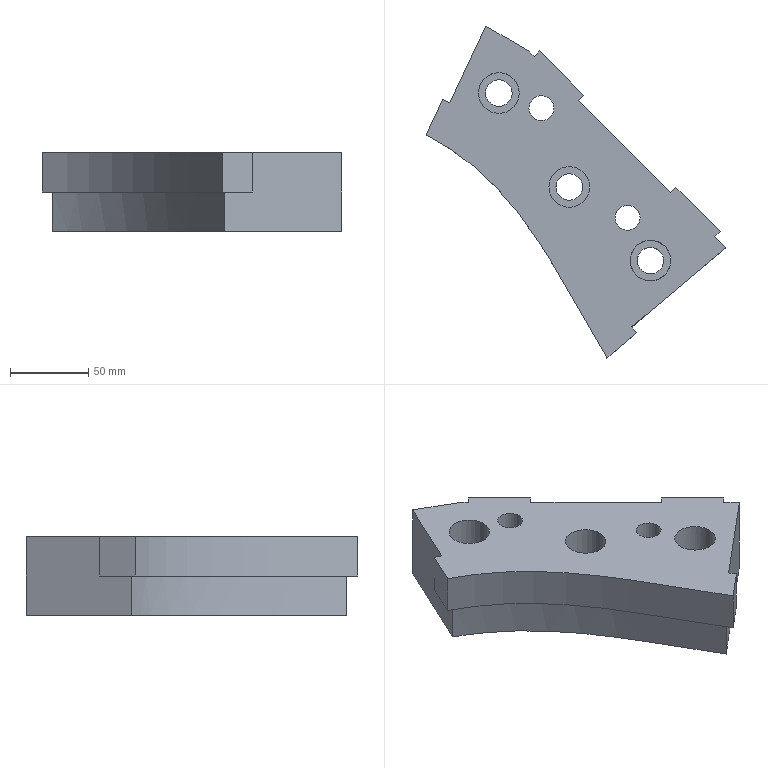Part | NX | features solid 2 | 1 solid | 32 faces | box 191.378 x 212.047 x 50 mm | volume 733271 mm3 | plane 22 | cylinder 8 | spline 2 | commonest cylinder face diameters 17 x3 26 x3 16 x2
STEP:
#1=CARTESIAN_POINT('',(8.245,-336.739,0.));
#2=VERTEX_POINT('',#1);
#3=CARTESIAN_POINT('',(1.173,-329.668,0.));
#4=VERTEX_POINT('',#3);
#5=CARTESIAN_POINT('',(11.794,-340.288,0.));
#6=DIRECTION('',(-0.7071,0.7071,0.));
#7=VECTOR('',#6,1000.);
#8=LINE('',#5,#7);
#9=EDGE_CURVE('',#2,#4,#8,.T.);
#10=ORIENTED_EDGE('',*,*,#9,.F.);
#11=CARTESIAN_POINT('',(8.245,-336.739,-50.));
#12=VERTEX_POINT('',#11);
#13=CARTESIAN_POINT('',(8.245,-336.739,-50.));
#14=DIRECTION('',(0.,0.,1.));
#15=VECTOR('',#14,1000.);
#16=LINE('',#13,#15);
#17=EDGE_CURVE('',#12,#2,#16,.T.);
#18=ORIENTED_EDGE('',*,*,#17,.F.);
#19=CARTESIAN_POINT('',(1.173,-329.668,-50.));
#20=VERTEX_POINT('',#19);
#21=CARTESIAN_POINT('',(11.794,-340.288,-50.));
#22=DIRECTION('',(-0.7071,0.7071,0.));
#23=VECTOR('',#22,1000.);
#24=LINE('',#21,#23);
#25=EDGE_CURVE('',#12,#20,#24,.T.);
#26=ORIENTED_EDGE('',*,*,#25,.T.);
#27=CARTESIAN_POINT('',(1.173,-329.668,-50.));
#28=DIRECTION('',(0.,0.,1.));
#29=VECTOR('',#28,1000.);
#30=LINE('',#27,#29);
#31=EDGE_CURVE('',#20,#4,#30,.T.);
#32=ORIENTED_EDGE('',*,*,#31,.T.);
#33=EDGE_LOOP('',(#10,#18,#26,#32));
#34=FACE_BOUND('',#33,.T.);
#35=CARTESIAN_POINT('',(11.794,-340.288,-50.));
#36=DIRECTION('',(0.7071,0.7071,0.));
#37=DIRECTION('',(-0.7071,0.7071,0.));
#38=AXIS2_PLACEMENT_3D('',#35,#36,#37);
#39=PLANE('',#38);
#40=ADVANCED_FACE('',(#34),#39,.T.);
#41=CARTESIAN_POINT('',(-48.541,-390.915,-25.));
#42=VERTEX_POINT('',#41);
#43=CARTESIAN_POINT('',(-51.755,-387.085,-25.));
#44=VERTEX_POINT('',#43);
#45=CARTESIAN_POINT('',(-45.327,-394.745,-25.));
#46=DIRECTION('',(-0.6428,0.766,0.));
#47=VECTOR('',#46,1000.);
#48=LINE('',#45,#47);
#49=EDGE_CURVE('',#42,#44,#48,.T.);
#50=ORIENTED_EDGE('',*,*,#49,.F.);
#51=CARTESIAN_POINT('',(-67.692,-406.985,-25.));
#52=VERTEX_POINT('',#51);
#53=CARTESIAN_POINT('',(-67.692,-406.985,-25.));
#54=DIRECTION('',(-0.766,-0.6428,0.));
#55=VECTOR('',#54,1000.);
#56=LINE('',#53,#55);
#57=EDGE_CURVE('',#42,#52,#56,.T.);
#58=ORIENTED_EDGE('',*,*,#57,.T.);
#59=CARTESIAN_POINT('',(-183.133,-264.552,-25.));
#60=VERTEX_POINT('',#59);
#61=CARTESIAN_POINT('',(-183.133,-264.552,-25.));
#62=CARTESIAN_POINT('',(-182.734,-264.756,-25.));
#63=CARTESIAN_POINT('',(-176.179,-268.157,-25.));
#64=CARTESIAN_POINT('',(-163.887,-275.581,-25.));
#65=CARTESIAN_POINT('',(-147.555,-288.567,-25.));
#66=CARTESIAN_POINT('',(-132.971,-303.448,-25.));
#67=CARTESIAN_POINT('',(-115.628,-325.186,-25.));
#68=CARTESIAN_POINT('',(-97.34,-354.727,-25.));
#69=CARTESIAN_POINT('',(-80.928,-384.396,-25.));
#70=CARTESIAN_POINT('',(-70.839,-401.701,-25.));
#71=CARTESIAN_POINT('',(-67.692,-406.985,-25.));
#72=B_SPLINE_CURVE_WITH_KNOTS('',3,(#61,#62,#63,#64,#65,#66,#67,#68,#69,#70,#71),.UNSPECIFIED.,.F.,.F.,(4,1,1,1,1,1,1,1,4),(0.,0.007224,0.1189,0.2307,0.3424,0.4541,0.6776,0.901,1.),.UNSPECIFIED.);
#73=EDGE_CURVE('',#52,#60,#72,.F.);
#74=ORIENTED_EDGE('',*,*,#73,.T.);
#75=CARTESIAN_POINT('',(-172.568,-241.894,-25.));
#76=VERTEX_POINT('',#75);
#77=CARTESIAN_POINT('',(-183.133,-264.552,-25.));
#78=DIRECTION('',(-0.4226,-0.9063,0.));
#79=VECTOR('',#78,1000.);
#80=LINE('',#77,#79);
#81=EDGE_CURVE('',#76,#60,#80,.T.);
#82=ORIENTED_EDGE('',*,*,#81,.F.);
#83=CARTESIAN_POINT('',(-168.036,-244.007,-25.));
#84=VERTEX_POINT('',#83);
#85=CARTESIAN_POINT('',(-177.099,-239.781,-25.));
#86=DIRECTION('',(0.9063,-0.4226,0.));
#87=VECTOR('',#86,1000.);
#88=LINE('',#85,#87);
#89=EDGE_CURVE('',#76,#84,#88,.T.);
#90=ORIENTED_EDGE('',*,*,#89,.T.);
#91=CARTESIAN_POINT('',(-176.596,-262.363,-25.));
#92=VERTEX_POINT('',#91);
#93=CARTESIAN_POINT('',(-178.602,-266.665,-25.));
#94=DIRECTION('',(-0.4226,-0.9063,0.));
#95=VECTOR('',#94,1000.);
#96=LINE('',#93,#95);
#97=EDGE_CURVE('',#92,#84,#96,.F.);
#98=ORIENTED_EDGE('',*,*,#97,.F.);
#99=CARTESIAN_POINT('',(-66.391,-399.365,-25.));
#100=VERTEX_POINT('',#99);
#101=CARTESIAN_POINT('',(-176.596,-262.363,-25.));
#102=CARTESIAN_POINT('',(-169.988,-265.991,-25.));
#103=CARTESIAN_POINT('',(-157.223,-274.12,-25.));
#104=CARTESIAN_POINT('',(-134.139,-293.687,-25.));
#105=CARTESIAN_POINT('',(-110.503,-323.019,-25.));
#106=CARTESIAN_POINT('',(-87.959,-361.257,-25.));
#107=CARTESIAN_POINT('',(-73.779,-386.798,-25.));
#108=CARTESIAN_POINT('',(-66.391,-399.365,-25.));
#109=B_SPLINE_CURVE_WITH_KNOTS('',3,(#101,#102,#103,#104,#105,#106,#107,#108),.UNSPECIFIED.,.F.,.F.,(4,1,1,1,1,4),(0.02511,0.143,0.2609,0.4967,0.7325,0.9683),.UNSPECIFIED.);
#110=EDGE_CURVE('',#92,#100,#109,.T.);
#111=ORIENTED_EDGE('',*,*,#110,.T.);
#112=CARTESIAN_POINT('',(-70.906,-403.154,-25.));
#113=DIRECTION('',(-0.766,-0.6428,0.));
#114=VECTOR('',#113,1000.);
#115=LINE('',#112,#114);
#116=EDGE_CURVE('',#100,#44,#115,.F.);
#117=ORIENTED_EDGE('',*,*,#116,.T.);
#118=EDGE_LOOP('',(#50,#58,#74,#82,#90,#98,#111,#117));
#119=FACE_BOUND('',#118,.T.);
#120=CARTESIAN_POINT('',(-56.169,-397.653,-25.));
#121=DIRECTION('',(0.,0.,-1.));
#122=DIRECTION('',(-1.,0.,0.));
#123=AXIS2_PLACEMENT_3D('',#120,#121,#122);
#124=PLANE('',#123);
#125=ADVANCED_FACE('',(#119),#124,.T.);
#126=CARTESIAN_POINT('',(-101.523,-247.421,0.));
#127=VERTEX_POINT('',#126);
#128=CARTESIAN_POINT('',(-109.523,-247.421,0.));
#129=DIRECTION('',(0.,0.,1.));
#130=DIRECTION('',(1.,0.,0.));
#131=AXIS2_PLACEMENT_3D('',#128,#129,#130);
#132=CIRCLE('',#131,8.);
#133=EDGE_CURVE('',#127,#127,#132,.T.);
#134=ORIENTED_EDGE('',*,*,#133,.F.);
#135=EDGE_LOOP('',(#134));
#136=FACE_BOUND('',#135,.T.);
#137=CARTESIAN_POINT('',(-46.523,-317.421,0.));
#138=VERTEX_POINT('',#137);
#139=CARTESIAN_POINT('',(-54.523,-317.421,0.));
#140=DIRECTION('',(0.,0.,1.));
#141=DIRECTION('',(1.,0.,0.));
#142=AXIS2_PLACEMENT_3D('',#139,#140,#141);
#143=CIRCLE('',#142,8.);
#144=EDGE_CURVE('',#138,#138,#143,.T.);
#145=ORIENTED_EDGE('',*,*,#144,.F.);
#146=EDGE_LOOP('',(#145));
#147=FACE_BOUND('',#146,.T.);
#148=CARTESIAN_POINT('',(-48.541,-390.915,0.));
#149=VERTEX_POINT('',#148);
#150=CARTESIAN_POINT('',(-51.755,-387.085,0.));
#151=VERTEX_POINT('',#150);
#152=CARTESIAN_POINT('',(-45.327,-394.745,0.));
#153=DIRECTION('',(-0.6428,0.766,0.));
#154=VECTOR('',#153,1000.);
#155=LINE('',#152,#154);
#156=EDGE_CURVE('',#149,#151,#155,.T.);
#157=ORIENTED_EDGE('',*,*,#156,.T.);
#158=CARTESIAN_POINT('',(-70.906,-403.154,0.));
#159=DIRECTION('',(0.766,0.6428,0.));
#160=VECTOR('',#159,1000.);
#161=LINE('',#158,#160);
#162=EDGE_CURVE('',#151,#2,#161,.T.);
#163=ORIENTED_EDGE('',*,*,#162,.T.);
#164=ORIENTED_EDGE('',*,*,#9,.T.);
#165=CARTESIAN_POINT('',(4.709,-326.132,0.));
#166=VERTEX_POINT('',#165);
#167=CARTESIAN_POINT('',(1.173,-329.668,0.));
#168=DIRECTION('',(0.7071,0.7071,0.));
#169=VECTOR('',#168,1000.);
#170=LINE('',#167,#169);
#171=EDGE_CURVE('',#4,#166,#170,.T.);
#172=ORIENTED_EDGE('',*,*,#171,.T.);
#173=CARTESIAN_POINT('',(-23.575,-297.848,0.));
#174=VERTEX_POINT('',#173);
#175=CARTESIAN_POINT('',(109.467,-430.891,0.));
#176=DIRECTION('',(-0.7071,0.7071,0.));
#177=VECTOR('',#176,1000.);
#178=LINE('',#175,#177);
#179=EDGE_CURVE('',#166,#174,#178,.T.);
#180=ORIENTED_EDGE('',*,*,#179,.T.);
#181=CARTESIAN_POINT('',(-27.111,-301.384,0.));
#182=VERTEX_POINT('',#181);
#183=CARTESIAN_POINT('',(-27.111,-301.384,0.));
#184=DIRECTION('',(0.7071,0.7071,0.));
#185=VECTOR('',#184,1000.);
#186=LINE('',#183,#185);
#187=EDGE_CURVE('',#182,#174,#186,.T.);
#188=ORIENTED_EDGE('',*,*,#187,.F.);
#189=CARTESIAN_POINT('',(-85.894,-242.601,0.));
#190=VERTEX_POINT('',#189);
#191=CARTESIAN_POINT('',(11.794,-340.288,0.));
#192=DIRECTION('',(-0.7071,0.7071,0.));
#193=VECTOR('',#192,1000.);
#194=LINE('',#191,#193);
#195=EDGE_CURVE('',#182,#190,#194,.T.);
#196=ORIENTED_EDGE('',*,*,#195,.T.);
#197=CARTESIAN_POINT('',(-82.358,-239.065,0.));
#198=VERTEX_POINT('',#197);
#199=CARTESIAN_POINT('',(-85.894,-242.601,0.));
#200=DIRECTION('',(0.7071,0.7071,0.));
#201=VECTOR('',#200,1000.);
#202=LINE('',#199,#201);
#203=EDGE_CURVE('',#190,#198,#202,.T.);
#204=ORIENTED_EDGE('',*,*,#203,.T.);
#205=CARTESIAN_POINT('',(-110.642,-210.781,0.));
#206=VERTEX_POINT('',#205);
#207=CARTESIAN_POINT('',(15.329,-336.753,0.));
#208=DIRECTION('',(-0.7071,0.7071,0.));
#209=VECTOR('',#208,1000.);
#210=LINE('',#207,#209);
#211=EDGE_CURVE('',#198,#206,#210,.T.);
#212=ORIENTED_EDGE('',*,*,#211,.T.);
#213=CARTESIAN_POINT('',(-114.178,-214.317,0.));
#214=VERTEX_POINT('',#213);
#215=CARTESIAN_POINT('',(-114.178,-214.317,0.));
#216=DIRECTION('',(0.7071,0.7071,0.));
#217=VECTOR('',#216,1000.);
#218=LINE('',#215,#217);
#219=EDGE_CURVE('',#214,#206,#218,.T.);
#220=ORIENTED_EDGE('',*,*,#219,.F.);
#221=CARTESIAN_POINT('',(-117.713,-210.781,0.));
#222=VERTEX_POINT('',#221);
#223=CARTESIAN_POINT('',(11.794,-340.288,0.));
#224=DIRECTION('',(-0.7071,0.7071,0.));
#225=VECTOR('',#224,1000.);
#226=LINE('',#223,#225);
#227=EDGE_CURVE('',#214,#222,#226,.T.);
#228=ORIENTED_EDGE('',*,*,#227,.T.);
#229=CARTESIAN_POINT('',(-145.155,-194.938,0.));
#230=VERTEX_POINT('',#229);
#231=CARTESIAN_POINT('',(-65.584,-240.878,0.));
#232=DIRECTION('',(-0.866,0.5,0.));
#233=VECTOR('',#232,1000.);
#234=LINE('',#231,#233);
#235=EDGE_CURVE('',#222,#230,#234,.T.);
#236=ORIENTED_EDGE('',*,*,#235,.T.);
#237=CARTESIAN_POINT('',(-168.036,-244.007,0.));
#238=VERTEX_POINT('',#237);
#239=CARTESIAN_POINT('',(-178.602,-266.665,0.));
#240=DIRECTION('',(0.4226,0.9063,0.));
#241=VECTOR('',#240,1000.);
#242=LINE('',#239,#241);
#243=EDGE_CURVE('',#238,#230,#242,.T.);
#244=ORIENTED_EDGE('',*,*,#243,.F.);
#245=CARTESIAN_POINT('',(-172.568,-241.894,0.));
#246=VERTEX_POINT('',#245);
#247=CARTESIAN_POINT('',(-177.099,-239.781,0.));
#248=DIRECTION('',(0.9063,-0.4226,0.));
#249=VECTOR('',#248,1000.);
#250=LINE('',#247,#249);
#251=EDGE_CURVE('',#246,#238,#250,.T.);
#252=ORIENTED_EDGE('',*,*,#251,.F.);
#253=CARTESIAN_POINT('',(-183.133,-264.552,0.));
#254=VERTEX_POINT('',#253);
#255=CARTESIAN_POINT('',(-183.133,-264.552,0.));
#256=DIRECTION('',(0.4226,0.9063,0.));
#257=VECTOR('',#256,1000.);
#258=LINE('',#255,#257);
#259=EDGE_CURVE('',#254,#246,#258,.T.);
#260=ORIENTED_EDGE('',*,*,#259,.F.);
#261=CARTESIAN_POINT('',(-67.692,-406.985,0.));
#262=VERTEX_POINT('',#261);
#263=CARTESIAN_POINT('',(-183.133,-264.552,0.));
#264=CARTESIAN_POINT('',(-182.734,-264.756,0.));
#265=CARTESIAN_POINT('',(-176.179,-268.157,0.));
#266=CARTESIAN_POINT('',(-163.887,-275.581,0.));
#267=CARTESIAN_POINT('',(-147.555,-288.567,0.));
#268=CARTESIAN_POINT('',(-132.971,-303.448,0.));
#269=CARTESIAN_POINT('',(-115.628,-325.186,0.));
#270=CARTESIAN_POINT('',(-97.34,-354.727,0.));
#271=CARTESIAN_POINT('',(-80.928,-384.396,0.));
#272=CARTESIAN_POINT('',(-70.839,-401.701,0.));
#273=CARTESIAN_POINT('',(-67.692,-406.985,0.));
#274=B_SPLINE_CURVE_WITH_KNOTS('',3,(#263,#264,#265,#266,#267,#268,#269,#270,#271,#272,#273),.UNSPECIFIED.,.F.,.F.,(4,1,1,1,1,1,1,1,4),(0.,0.007224,0.1189,0.2307,0.3424,0.4541,0.6776,0.901,1.),.UNSPECIFIED.);
#275=EDGE_CURVE('',#254,#262,#274,.T.);
#276=ORIENTED_EDGE('',*,*,#275,.T.);
#277=CARTESIAN_POINT('',(-67.692,-406.985,0.));
#278=DIRECTION('',(0.766,0.6428,0.));
#279=VECTOR('',#278,1000.);
#280=LINE('',#277,#279);
#281=EDGE_CURVE('',#262,#149,#280,.T.);
#282=ORIENTED_EDGE('',*,*,#281,.T.);
#283=EDGE_LOOP('',(#157,#163,#164,#172,#180,#188,#196,#204,#212,#220,#228,#236,#244,#252,#260,#276,#282));
#284=FACE_BOUND('',#283,.T.);
#285=CARTESIAN_POINT('',(-78.729,-297.741,0.));
#286=VERTEX_POINT('',#285);
#287=CARTESIAN_POINT('',(-91.729,-297.741,0.));
#288=DIRECTION('',(0.,0.,1.));
#289=DIRECTION('',(1.,0.,0.));
#290=AXIS2_PLACEMENT_3D('',#287,#288,#289);
#291=CIRCLE('',#290,13.);
#292=EDGE_CURVE('',#286,#286,#291,.T.);
#293=ORIENTED_EDGE('',*,*,#292,.F.);
#294=EDGE_LOOP('',(#293));
#295=FACE_BOUND('',#294,.T.);
#296=CARTESIAN_POINT('',(-26.878,-344.794,0.));
#297=VERTEX_POINT('',#296);
#298=CARTESIAN_POINT('',(-39.878,-344.794,0.));
#299=DIRECTION('',(0.,0.,1.));
#300=DIRECTION('',(1.,0.,0.));
#301=AXIS2_PLACEMENT_3D('',#298,#299,#300);
#302=CIRCLE('',#301,13.);
#303=EDGE_CURVE('',#297,#297,#302,.T.);
#304=ORIENTED_EDGE('',*,*,#303,.F.);
#305=EDGE_LOOP('',(#304));
#306=FACE_BOUND('',#305,.T.);
#307=CARTESIAN_POINT('',(-123.729,-237.741,0.));
#308=VERTEX_POINT('',#307);
#309=CARTESIAN_POINT('',(-136.729,-237.741,0.));
#310=DIRECTION('',(0.,0.,1.));
#311=DIRECTION('',(1.,0.,0.));
#312=AXIS2_PLACEMENT_3D('',#309,#310,#311);
#313=CIRCLE('',#312,13.);
#314=EDGE_CURVE('',#308,#308,#313,.T.);
#315=ORIENTED_EDGE('',*,*,#314,.F.);
#316=EDGE_LOOP('',(#315));
#317=FACE_BOUND('',#316,.T.);
#318=CARTESIAN_POINT('',(-557.805,-998.377,0.));
#319=DIRECTION('',(0.,0.,1.));
#320=DIRECTION('',(1.,0.,0.));
#321=AXIS2_PLACEMENT_3D('',#318,#319,#320);
#322=PLANE('',#321);
#323=ADVANCED_FACE('',(#136,#147,#284,#295,#306,#317),#322,.T.);
#324=CARTESIAN_POINT('',(-172.568,-241.894,-50.));
#325=DIRECTION('',(0.,0.,1.));
#326=VECTOR('',#325,1000.);
#327=LINE('',#324,#326);
#328=EDGE_CURVE('',#76,#246,#327,.T.);
#329=ORIENTED_EDGE('',*,*,#328,.F.);
#330=ORIENTED_EDGE('',*,*,#81,.T.);
#331=CARTESIAN_POINT('',(-183.133,-264.552,-50.));
#332=DIRECTION('',(0.,0.,1.));
#333=VECTOR('',#332,1000.);
#334=LINE('',#331,#333);
#335=EDGE_CURVE('',#60,#254,#334,.T.);
#336=ORIENTED_EDGE('',*,*,#335,.T.);
#337=ORIENTED_EDGE('',*,*,#259,.T.);
#338=EDGE_LOOP('',(#329,#330,#336,#337));
#339=FACE_BOUND('',#338,.T.);
#340=CARTESIAN_POINT('',(-183.133,-264.552,-50.));
#341=DIRECTION('',(0.9063,-0.4226,0.));
#342=DIRECTION('',(0.4226,0.9063,0.));
#343=AXIS2_PLACEMENT_3D('',#340,#341,#342);
#344=PLANE('',#343);
#345=ADVANCED_FACE('',(#339),#344,.F.);
#346=CARTESIAN_POINT('',(-101.523,-247.421,-50.));
#347=VERTEX_POINT('',#346);
#348=CARTESIAN_POINT('',(-109.523,-247.421,-50.));
#349=DIRECTION('',(0.,0.,1.));
#350=DIRECTION('',(1.,0.,0.));
#351=AXIS2_PLACEMENT_3D('',#348,#349,#350);
#352=CIRCLE('',#351,8.);
#353=EDGE_CURVE('',#347,#347,#352,.T.);
#354=ORIENTED_EDGE('',*,*,#353,.T.);
#355=EDGE_LOOP('',(#354));
#356=FACE_BOUND('',#355,.T.);
#357=CARTESIAN_POINT('',(-46.523,-317.421,-50.));
#358=VERTEX_POINT('',#357);
#359=CARTESIAN_POINT('',(-54.523,-317.421,-50.));
#360=DIRECTION('',(0.,0.,1.));
#361=DIRECTION('',(1.,0.,0.));
#362=AXIS2_PLACEMENT_3D('',#359,#360,#361);
#363=CIRCLE('',#362,8.);
#364=EDGE_CURVE('',#358,#358,#363,.T.);
#365=ORIENTED_EDGE('',*,*,#364,.T.);
#366=EDGE_LOOP('',(#365));
#367=FACE_BOUND('',#366,.T.);
#368=CARTESIAN_POINT('',(-128.229,-237.741,-50.));
#369=VERTEX_POINT('',#368);
#370=CARTESIAN_POINT('',(-136.729,-237.741,-50.));
#371=DIRECTION('',(0.,0.,1.));
#372=DIRECTION('',(1.,0.,0.));
#373=AXIS2_PLACEMENT_3D('',#370,#371,#372);
#374=CIRCLE('',#373,8.5);
#375=EDGE_CURVE('',#369,#369,#374,.T.);
#376=ORIENTED_EDGE('',*,*,#375,.T.);
#377=EDGE_LOOP('',(#376));
#378=FACE_BOUND('',#377,.T.);
#379=ORIENTED_EDGE('',*,*,#25,.F.);
#380=CARTESIAN_POINT('',(-66.391,-399.365,-50.));
#381=VERTEX_POINT('',#380);
#382=CARTESIAN_POINT('',(-59.36,-393.466,-50.));
#383=DIRECTION('',(-0.766,-0.6428,0.));
#384=VECTOR('',#383,1000.);
#385=LINE('',#382,#384);
#386=EDGE_CURVE('',#12,#381,#385,.T.);
#387=ORIENTED_EDGE('',*,*,#386,.T.);
#388=CARTESIAN_POINT('',(-176.596,-262.363,-50.));
#389=VERTEX_POINT('',#388);
#390=CARTESIAN_POINT('',(-66.391,-399.365,-50.));
#391=CARTESIAN_POINT('',(-67.194,-397.999,-50.));
#392=CARTESIAN_POINT('',(-68.864,-395.141,-50.));
#393=CARTESIAN_POINT('',(-71.109,-391.26,-50.));
#394=CARTESIAN_POINT('',(-73.001,-387.969,-50.));
#395=CARTESIAN_POINT('',(-74.222,-385.835,-50.));
#396=CARTESIAN_POINT('',(-75.223,-384.08,-50.));
#397=CARTESIAN_POINT('',(-75.984,-382.743,-50.));
#398=CARTESIAN_POINT('',(-76.633,-381.601,-50.));
#399=CARTESIAN_POINT('',(-77.082,-380.81,-50.));
#400=CARTESIAN_POINT('',(-77.357,-380.325,-50.));
#401=CARTESIAN_POINT('',(-77.517,-380.043,-50.));
#402=CARTESIAN_POINT('',(-77.857,-379.443,-50.));
#403=CARTESIAN_POINT('',(-78.241,-378.766,-50.));
#404=CARTESIAN_POINT('',(-78.929,-377.553,-50.));
#405=CARTESIAN_POINT('',(-79.854,-375.92,-50.));
#406=CARTESIAN_POINT('',(-80.906,-374.065,-50.));
#407=CARTESIAN_POINT('',(-82.219,-371.751,-50.));
#408=CARTESIAN_POINT('',(-83.697,-369.146,-50.));
#409=CARTESIAN_POINT('',(-85.208,-366.484,-50.));
#410=CARTESIAN_POINT('',(-86.457,-364.285,-50.));
#411=CARTESIAN_POINT('',(-87.278,-362.839,-50.));
#412=CARTESIAN_POINT('',(-87.805,-361.914,-50.));
#413=CARTESIAN_POINT('',(-88.079,-361.433,-50.));
#414=CARTESIAN_POINT('',(-88.266,-361.105,-50.));
#415=CARTESIAN_POINT('',(-88.389,-360.89,-50.));
#416=CARTESIAN_POINT('',(-88.482,-360.728,-50.));
#417=CARTESIAN_POINT('',(-88.531,-360.641,-50.));
#418=CARTESIAN_POINT('',(-88.57,-360.573,-50.));
#419=CARTESIAN_POINT('',(-88.562,-360.587,-50.));
#420=CARTESIAN_POINT('',(-88.692,-360.361,-50.));
#421=CARTESIAN_POINT('',(-88.816,-360.145,-50.));
#422=CARTESIAN_POINT('',(-89.055,-359.728,-50.));
#423=CARTESIAN_POINT('',(-89.384,-359.157,-50.));
#424=CARTESIAN_POINT('',(-89.78,-358.47,-50.));
#425=CARTESIAN_POINT('',(-90.302,-357.564,-50.));
#426=CARTESIAN_POINT('',(-90.948,-356.447,-50.));
#427=CARTESIAN_POINT('',(-91.965,-354.693,-50.));
#428=CARTESIAN_POINT('',(-93.208,-352.563,-50.));
#429=CARTESIAN_POINT('',(-95.133,-349.288,-50.));
#430=CARTESIAN_POINT('',(-96.96,-346.217,-50.));
#431=CARTESIAN_POINT('',(-98.483,-343.694,-50.));
#432=CARTESIAN_POINT('',(-99.214,-342.491,-50.));
#433=CARTESIAN_POINT('',(-99.641,-341.793,-50.));
#434=CARTESIAN_POINT('',(-99.917,-341.341,-50.));
#435=CARTESIAN_POINT('',(-100.346,-340.644,-50.));
#436=CARTESIAN_POINT('',(-100.862,-339.806,-50.));
#437=CARTESIAN_POINT('',(-101.787,-338.313,-50.));
#438=CARTESIAN_POINT('',(-103.086,-336.24,-50.));
#439=CARTESIAN_POINT('',(-104.635,-333.804,-50.));
#440=CARTESIAN_POINT('',(-106.677,-330.643,-50.));
#441=CARTESIAN_POINT('',(-108.693,-327.596,-50.));
#442=CARTESIAN_POINT('',(-110.416,-325.058,-50.));
#443=CARTESIAN_POINT('',(-111.414,-323.609,-50.));
#444=CARTESIAN_POINT('',(-112.1,-322.621,-50.));
#445=CARTESIAN_POINT('',(-113.008,-321.327,-50.));
#446=CARTESIAN_POINT('',(-114.144,-319.727,-50.));
#447=CARTESIAN_POINT('',(-116.175,-316.913,-50.));
#448=CARTESIAN_POINT('',(-119.077,-313.029,-50.));
#449=CARTESIAN_POINT('',(-122.6,-308.531,-50.));
#450=CARTESIAN_POINT('',(-127.337,-302.772,-50.));
#451=CARTESIAN_POINT('',(-132.146,-297.353,-50.));
#452=CARTESIAN_POINT('',(-136.39,-292.937,-50.));
#453=CARTESIAN_POINT('',(-138.862,-290.471,-50.));
#454=CARTESIAN_POINT('',(-140.637,-288.747,-50.));
#455=CARTESIAN_POINT('',(-142.751,-286.755,-50.));
#456=CARTESIAN_POINT('',(-145.495,-284.257,-50.));
#457=CARTESIAN_POINT('',(-150.44,-279.965,-50.));
#458=CARTESIAN_POINT('',(-157.739,-274.235,-50.));
#459=CARTESIAN_POINT('',(-166.925,-267.948,-50.));
#460=CARTESIAN_POINT('',(-173.326,-264.158,-50.));
#461=CARTESIAN_POINT('',(-176.596,-262.363,-50.));
#462=B_SPLINE_CURVE_WITH_KNOTS('',3,(#390,#391,#392,#393,#394,#395,#396,#397,#398,#399,#400,#401,#402,#403,#404,#405,#406,#407,#408,#409,#410,#411,#412,#413,#414,#415,#416,#417,#418,#419,#420,#421,#422,#423,#424,#425,#426,#427,#428,#429,#430,#431,#432,#433,#434,#435,#436,#437,#438,#439,#440,#441,#442,#443,#444,#445,#446,#447,#448,#449,#450,#451,#452,#453,#454,#455,#456,#457,#458,#459,#460,#461),.UNSPECIFIED.,.F.,.F.,(4,1,1,1,1,1,1,1,1,1,1,1,1,1,1,1,1,1,1,1,1,1,1,1,1,1,1,1,1,1,1,1,1,1,1,1,1,1,1,1,1,1,1,1,1,1,1,1,1,1,1,1,1,1,1,1,1,1,1,1,1,1,1,1,1,1,1,1,1,4),(0.,0.03125,0.0625,0.07812,0.09375,0.1016,0.1094,0.1172,0.1211,0.123,0.125,0.127,0.1289,0.1328,0.1406,0.1484,0.1562,0.1719,0.1875,0.2031,0.2188,0.2266,0.2344,0.2383,0.2422,0.2461,0.248,0.249,0.25,0.251,0.252,0.2539,0.2578,0.2617,0.2656,0.2734,0.2812,0.2969,0.3125,0.3438,0.3594,0.3672,0.3711,0.375,0.3789,0.3828,0.3906,0.4062,0.4219,0.4375,0.4688,0.4844,0.4922,0.5,0.5078,0.5156,0.5312,0.5625,0.5938,0.625,0.6875,0.7188,0.7344,0.75,0.7656,0.7812,0.8125,0.875,0.9375,1.),.UNSPECIFIED.);
#463=EDGE_CURVE('',#381,#389,#462,.T.);
#464=ORIENTED_EDGE('',*,*,#463,.T.);
#465=CARTESIAN_POINT('',(-145.155,-194.938,-50.));
#466=VERTEX_POINT('',#465);
#467=CARTESIAN_POINT('',(-190.347,-291.852,-50.));
#468=DIRECTION('',(-0.4226,-0.9063,0.));
#469=VECTOR('',#468,1000.);
#470=LINE('',#467,#469);
#471=EDGE_CURVE('',#466,#389,#470,.T.);
#472=ORIENTED_EDGE('',*,*,#471,.F.);
#473=CARTESIAN_POINT('',(-117.713,-210.781,-50.));
#474=VERTEX_POINT('',#473);
#475=CARTESIAN_POINT('',(-65.584,-240.878,-50.));
#476=DIRECTION('',(-0.866,0.5,0.));
#477=VECTOR('',#476,1000.);
#478=LINE('',#475,#477);
#479=EDGE_CURVE('',#474,#466,#478,.T.);
#480=ORIENTED_EDGE('',*,*,#479,.F.);
#481=CARTESIAN_POINT('',(-114.178,-214.317,-50.));
#482=VERTEX_POINT('',#481);
#483=CARTESIAN_POINT('',(11.794,-340.288,-50.));
#484=DIRECTION('',(-0.7071,0.7071,0.));
#485=VECTOR('',#484,1000.);
#486=LINE('',#483,#485);
#487=EDGE_CURVE('',#482,#474,#486,.T.);
#488=ORIENTED_EDGE('',*,*,#487,.F.);
#489=CARTESIAN_POINT('',(-110.642,-210.781,-50.));
#490=VERTEX_POINT('',#489);
#491=CARTESIAN_POINT('',(-114.178,-214.317,-50.));
#492=DIRECTION('',(0.7071,0.7071,0.));
#493=VECTOR('',#492,1000.);
#494=LINE('',#491,#493);
#495=EDGE_CURVE('',#482,#490,#494,.T.);
#496=ORIENTED_EDGE('',*,*,#495,.T.);
#497=CARTESIAN_POINT('',(-82.358,-239.065,-50.));
#498=VERTEX_POINT('',#497);
#499=CARTESIAN_POINT('',(15.329,-336.753,-50.));
#500=DIRECTION('',(-0.7071,0.7071,0.));
#501=VECTOR('',#500,1000.);
#502=LINE('',#499,#501);
#503=EDGE_CURVE('',#498,#490,#502,.T.);
#504=ORIENTED_EDGE('',*,*,#503,.F.);
#505=CARTESIAN_POINT('',(-85.894,-242.601,-50.));
#506=VERTEX_POINT('',#505);
#507=CARTESIAN_POINT('',(-85.894,-242.601,-50.));
#508=DIRECTION('',(0.7071,0.7071,0.));
#509=VECTOR('',#508,1000.);
#510=LINE('',#507,#509);
#511=EDGE_CURVE('',#506,#498,#510,.T.);
#512=ORIENTED_EDGE('',*,*,#511,.F.);
#513=CARTESIAN_POINT('',(-27.111,-301.384,-50.));
#514=VERTEX_POINT('',#513);
#515=CARTESIAN_POINT('',(11.794,-340.288,-50.));
#516=DIRECTION('',(-0.7071,0.7071,0.));
#517=VECTOR('',#516,1000.);
#518=LINE('',#515,#517);
#519=EDGE_CURVE('',#514,#506,#518,.T.);
#520=ORIENTED_EDGE('',*,*,#519,.F.);
#521=CARTESIAN_POINT('',(-23.575,-297.848,-50.));
#522=VERTEX_POINT('',#521);
#523=CARTESIAN_POINT('',(-27.111,-301.384,-50.));
#524=DIRECTION('',(0.7071,0.7071,0.));
#525=VECTOR('',#524,1000.);
#526=LINE('',#523,#525);
#527=EDGE_CURVE('',#514,#522,#526,.T.);
#528=ORIENTED_EDGE('',*,*,#527,.T.);
#529=CARTESIAN_POINT('',(4.709,-326.132,-50.));
#530=VERTEX_POINT('',#529);
#531=CARTESIAN_POINT('',(109.467,-430.891,-50.));
#532=DIRECTION('',(-0.7071,0.7071,0.));
#533=VECTOR('',#532,1000.);
#534=LINE('',#531,#533);
#535=EDGE_CURVE('',#530,#522,#534,.T.);
#536=ORIENTED_EDGE('',*,*,#535,.F.);
#537=CARTESIAN_POINT('',(1.173,-329.668,-50.));
#538=DIRECTION('',(0.7071,0.7071,0.));
#539=VECTOR('',#538,1000.);
#540=LINE('',#537,#539);
#541=EDGE_CURVE('',#20,#530,#540,.T.);
#542=ORIENTED_EDGE('',*,*,#541,.F.);
#543=EDGE_LOOP('',(#379,#387,#464,#472,#480,#488,#496,#504,#512,#520,#528,#536,#542));
#544=FACE_BOUND('',#543,.T.);
#545=CARTESIAN_POINT('',(-31.378,-344.794,-50.));
#546=VERTEX_POINT('',#545);
#547=CARTESIAN_POINT('',(-39.878,-344.794,-50.));
#548=DIRECTION('',(0.,0.,1.));
#549=DIRECTION('',(1.,0.,0.));
#550=AXIS2_PLACEMENT_3D('',#547,#548,#549);
#551=CIRCLE('',#550,8.5);
#552=EDGE_CURVE('',#546,#546,#551,.T.);
#553=ORIENTED_EDGE('',*,*,#552,.T.);
#554=EDGE_LOOP('',(#553));
#555=FACE_BOUND('',#554,.T.);
#556=CARTESIAN_POINT('',(-83.229,-297.741,-50.));
#557=VERTEX_POINT('',#556);
#558=CARTESIAN_POINT('',(-91.729,-297.741,-50.));
#559=DIRECTION('',(0.,0.,1.));
#560=DIRECTION('',(1.,0.,0.));
#561=AXIS2_PLACEMENT_3D('',#558,#559,#560);
#562=CIRCLE('',#561,8.5);
#563=EDGE_CURVE('',#557,#557,#562,.T.);
#564=ORIENTED_EDGE('',*,*,#563,.T.);
#565=EDGE_LOOP('',(#564));
#566=FACE_BOUND('',#565,.T.);
#567=CARTESIAN_POINT('',(-557.805,-998.377,-50.));
#568=DIRECTION('',(0.,0.,1.));
#569=DIRECTION('',(1.,0.,0.));
#570=AXIS2_PLACEMENT_3D('',#567,#568,#569);
#571=PLANE('',#570);
#572=ADVANCED_FACE('',(#356,#367,#378,#544,#555,#566),#571,.F.);
#573=ORIENTED_EDGE('',*,*,#552,.F.);
#574=EDGE_LOOP('',(#573));
#575=FACE_BOUND('',#574,.T.);
#576=CARTESIAN_POINT('',(-39.878,-336.294,-25.));
#577=VERTEX_POINT('',#576);
#578=CARTESIAN_POINT('',(-39.878,-344.794,-25.));
#579=DIRECTION('',(0.,0.,-1.));
#580=DIRECTION('',(0.,1.,0.));
#581=AXIS2_PLACEMENT_3D('',#578,#579,#580);
#582=CIRCLE('',#581,8.5);
#583=EDGE_CURVE('',#577,#577,#582,.F.);
#584=ORIENTED_EDGE('',*,*,#583,.T.);
#585=EDGE_LOOP('',(#584));
#586=FACE_BOUND('',#585,.T.);
#587=CARTESIAN_POINT('',(-39.878,-344.794,-75.));
#588=DIRECTION('',(0.,0.,1.));
#589=DIRECTION('',(0.,-1.,0.));
#590=AXIS2_PLACEMENT_3D('',#587,#588,#589);
#591=CYLINDRICAL_SURFACE('',#590,8.5);
#592=ADVANCED_FACE('',(#575,#586),#591,.F.);
#593=CARTESIAN_POINT('',(-39.878,-357.794,-25.));
#594=VERTEX_POINT('',#593);
#595=CARTESIAN_POINT('',(-39.878,-344.794,-25.));
#596=DIRECTION('',(0.,0.,1.));
#597=DIRECTION('',(0.,-1.,0.));
#598=AXIS2_PLACEMENT_3D('',#595,#596,#597);
#599=CIRCLE('',#598,13.);
#600=EDGE_CURVE('',#594,#594,#599,.T.);
#601=ORIENTED_EDGE('',*,*,#600,.F.);
#602=EDGE_LOOP('',(#601));
#603=FACE_BOUND('',#602,.T.);
#604=ORIENTED_EDGE('',*,*,#303,.T.);
#605=EDGE_LOOP('',(#604));
#606=FACE_BOUND('',#605,.T.);
#607=CARTESIAN_POINT('',(-39.878,-344.794,-25.));
#608=DIRECTION('',(0.,0.,1.));
#609=DIRECTION('',(0.,-1.,0.));
#610=AXIS2_PLACEMENT_3D('',#607,#608,#609);
#611=CYLINDRICAL_SURFACE('',#610,13.);
#612=ADVANCED_FACE('',(#603,#606),#611,.F.);
#613=ORIENTED_EDGE('',*,*,#583,.F.);
#614=EDGE_LOOP('',(#613));
#615=FACE_BOUND('',#614,.T.);
#616=ORIENTED_EDGE('',*,*,#600,.T.);
#617=EDGE_LOOP('',(#616));
#618=FACE_BOUND('',#617,.T.);
#619=CARTESIAN_POINT('',(-39.878,-344.794,-25.));
#620=DIRECTION('',(0.,0.,-1.));
#621=DIRECTION('',(0.,1.,0.));
#622=AXIS2_PLACEMENT_3D('',#619,#620,#621);
#623=PLANE('',#622);
#624=ADVANCED_FACE('',(#615,#618),#623,.F.);
#625=ORIENTED_EDGE('',*,*,#116,.F.);
#626=CARTESIAN_POINT('',(-66.391,-399.365,-37.5));
#627=DIRECTION('',(0.,0.,-1.));
#628=VECTOR('',#627,1000.);
#629=LINE('',#626,#628);
#630=EDGE_CURVE('',#381,#100,#629,.F.);
#631=ORIENTED_EDGE('',*,*,#630,.F.);
#632=ORIENTED_EDGE('',*,*,#386,.F.);
#633=ORIENTED_EDGE('',*,*,#17,.T.);
#634=ORIENTED_EDGE('',*,*,#162,.F.);
#635=CARTESIAN_POINT('',(-51.755,-387.085,-50.));
#636=DIRECTION('',(0.,0.,1.));
#637=VECTOR('',#636,1000.);
#638=LINE('',#635,#637);
#639=EDGE_CURVE('',#44,#151,#638,.T.);
#640=ORIENTED_EDGE('',*,*,#639,.F.);
#641=EDGE_LOOP('',(#625,#631,#632,#633,#634,#640));
#642=FACE_BOUND('',#641,.T.);
#643=CARTESIAN_POINT('',(-70.906,-403.154,-25.));
#644=DIRECTION('',(-0.6428,0.766,0.));
#645=DIRECTION('',(-0.766,-0.6428,0.));
#646=AXIS2_PLACEMENT_3D('',#643,#644,#645);
#647=PLANE('',#646);
#648=ADVANCED_FACE('',(#642),#647,.F.);
#649=CARTESIAN_POINT('',(-48.541,-390.915,-50.));
#650=DIRECTION('',(0.,0.,-1.));
#651=VECTOR('',#650,1000.);
#652=LINE('',#649,#651);
#653=EDGE_CURVE('',#149,#42,#652,.T.);
#654=ORIENTED_EDGE('',*,*,#653,.F.);
#655=ORIENTED_EDGE('',*,*,#281,.F.);
#656=CARTESIAN_POINT('',(-67.692,-406.985,-50.));
#657=DIRECTION('',(0.,0.,1.));
#658=VECTOR('',#657,1000.);
#659=LINE('',#656,#658);
#660=EDGE_CURVE('',#52,#262,#659,.T.);
#661=ORIENTED_EDGE('',*,*,#660,.F.);
#662=ORIENTED_EDGE('',*,*,#57,.F.);
#663=EDGE_LOOP('',(#654,#655,#661,#662));
#664=FACE_BOUND('',#663,.T.);
#665=CARTESIAN_POINT('',(-67.692,-406.985,-50.));
#666=DIRECTION('',(0.6428,-0.766,0.));
#667=DIRECTION('',(0.766,0.6428,0.));
#668=AXIS2_PLACEMENT_3D('',#665,#666,#667);
#669=PLANE('',#668);
#670=ADVANCED_FACE('',(#664),#669,.T.);
#671=ORIENTED_EDGE('',*,*,#73,.F.);
#672=ORIENTED_EDGE('',*,*,#660,.T.);
#673=ORIENTED_EDGE('',*,*,#275,.F.);
#674=ORIENTED_EDGE('',*,*,#335,.F.);
#675=EDGE_LOOP('',(#671,#672,#673,#674));
#676=FACE_BOUND('',#675,.T.);
#677=CARTESIAN_POINT('',(-183.133,-264.552,-25.));
#678=CARTESIAN_POINT('',(-183.133,-264.552,0.));
#679=CARTESIAN_POINT('',(-176.23,-268.098,-25.));
#680=CARTESIAN_POINT('',(-176.23,-268.098,0.));
#681=CARTESIAN_POINT('',(-162.895,-276.137,-25.));
#682=CARTESIAN_POINT('',(-162.895,-276.137,0.));
#683=CARTESIAN_POINT('',(-138.806,-295.879,-25.));
#684=CARTESIAN_POINT('',(-138.806,-295.879,0.));
#685=CARTESIAN_POINT('',(-114.232,-326.233,-25.));
#686=CARTESIAN_POINT('',(-114.232,-326.233,0.));
#687=CARTESIAN_POINT('',(-90.759,-366.521,-25.));
#688=CARTESIAN_POINT('',(-90.759,-366.521,0.));
#689=CARTESIAN_POINT('',(-75.639,-393.643,-25.));
#690=CARTESIAN_POINT('',(-75.639,-393.643,0.));
#691=CARTESIAN_POINT('',(-67.692,-406.985,-25.));
#692=CARTESIAN_POINT('',(-67.692,-406.985,0.));
#693=B_SPLINE_SURFACE_WITH_KNOTS('',3,1,((#677,#678),(#679,#680),(#681,#682),(#683,#684),(#685,#686),(#687,#688),(#689,#690),(#691,#692)),.SURF_OF_LINEAR_EXTRUSION.,.F.,.F.,.F.,(4,1,1,1,1,4),(2,2),(0.,0.125,0.25,0.5,0.75,1.),(0.,1.),.UNSPECIFIED.);
#694=ADVANCED_FACE('',(#676),#693,.T.);
#695=ORIENTED_EDGE('',*,*,#463,.F.);
#696=ORIENTED_EDGE('',*,*,#630,.T.);
#697=ORIENTED_EDGE('',*,*,#110,.F.);
#698=CARTESIAN_POINT('',(-176.596,-262.363,-37.5));
#699=DIRECTION('',(0.,0.,-1.));
#700=VECTOR('',#699,1000.);
#701=LINE('',#698,#700);
#702=EDGE_CURVE('',#389,#92,#701,.F.);
#703=ORIENTED_EDGE('',*,*,#702,.F.);
#704=EDGE_LOOP('',(#695,#696,#697,#703));
#705=FACE_BOUND('',#704,.T.);
#706=CARTESIAN_POINT('',(-176.596,-262.363,-25.));
#707=CARTESIAN_POINT('',(-176.596,-262.363,-50.));
#708=CARTESIAN_POINT('',(-169.988,-265.991,-25.));
#709=CARTESIAN_POINT('',(-169.988,-265.991,-50.));
#710=CARTESIAN_POINT('',(-157.223,-274.12,-25.));
#711=CARTESIAN_POINT('',(-157.223,-274.12,-50.));
#712=CARTESIAN_POINT('',(-134.139,-293.687,-25.));
#713=CARTESIAN_POINT('',(-134.139,-293.687,-50.));
#714=CARTESIAN_POINT('',(-110.503,-323.019,-25.));
#715=CARTESIAN_POINT('',(-110.503,-323.019,-50.));
#716=CARTESIAN_POINT('',(-87.959,-361.257,-25.));
#717=CARTESIAN_POINT('',(-87.959,-361.257,-50.));
#718=CARTESIAN_POINT('',(-73.779,-386.798,-25.));
#719=CARTESIAN_POINT('',(-73.779,-386.798,-50.));
#720=CARTESIAN_POINT('',(-66.391,-399.365,-25.));
#721=CARTESIAN_POINT('',(-66.391,-399.365,-50.));
#722=B_SPLINE_SURFACE_WITH_KNOTS('',3,1,((#706,#707),(#708,#709),(#710,#711),(#712,#713),(#714,#715),(#716,#717),(#718,#719),(#720,#721)),.SURF_OF_LINEAR_EXTRUSION.,.F.,.F.,.F.,(4,1,1,1,1,4),(2,2),(0.02511,0.143,0.2609,0.4967,0.7325,0.9683),(0.,1.),.UNSPECIFIED.);
#723=ADVANCED_FACE('',(#705),#722,.F.);
#724=ORIENTED_EDGE('',*,*,#97,.T.);
#725=CARTESIAN_POINT('',(-168.036,-244.007,-50.));
#726=DIRECTION('',(0.,0.,1.));
#727=VECTOR('',#726,1000.);
#728=LINE('',#725,#727);
#729=EDGE_CURVE('',#84,#238,#728,.T.);
#730=ORIENTED_EDGE('',*,*,#729,.T.);
#731=ORIENTED_EDGE('',*,*,#243,.T.);
#732=CARTESIAN_POINT('',(-145.155,-194.938,-25.));
#733=DIRECTION('',(0.,0.,-1.));
#734=VECTOR('',#733,1000.);
#735=LINE('',#732,#734);
#736=EDGE_CURVE('',#230,#466,#735,.T.);
#737=ORIENTED_EDGE('',*,*,#736,.T.);
#738=ORIENTED_EDGE('',*,*,#471,.T.);
#739=ORIENTED_EDGE('',*,*,#702,.T.);
#740=EDGE_LOOP('',(#724,#730,#731,#737,#738,#739));
#741=FACE_BOUND('',#740,.T.);
#742=CARTESIAN_POINT('',(-178.602,-266.665,-25.));
#743=DIRECTION('',(-0.9063,0.4226,0.));
#744=DIRECTION('',(-0.4226,-0.9063,0.));
#745=AXIS2_PLACEMENT_3D('',#742,#743,#744);
#746=PLANE('',#745);
#747=ADVANCED_FACE('',(#741),#746,.T.);
#748=CARTESIAN_POINT('',(-123.729,-237.741,-25.));
#749=VERTEX_POINT('',#748);
#750=CARTESIAN_POINT('',(-136.729,-237.741,-25.));
#751=DIRECTION('',(0.,0.,1.));
#752=DIRECTION('',(1.,0.,0.));
#753=AXIS2_PLACEMENT_3D('',#750,#751,#752);
#754=CIRCLE('',#753,13.);
#755=EDGE_CURVE('',#749,#749,#754,.T.);
#756=ORIENTED_EDGE('',*,*,#755,.F.);
#757=EDGE_LOOP('',(#756));
#758=FACE_BOUND('',#757,.T.);
#759=ORIENTED_EDGE('',*,*,#314,.T.);
#760=EDGE_LOOP('',(#759));
#761=FACE_BOUND('',#760,.T.);
#762=CARTESIAN_POINT('',(-136.729,-237.741,-25.));
#763=DIRECTION('',(0.,0.,1.));
#764=DIRECTION('',(1.,0.,0.));
#765=AXIS2_PLACEMENT_3D('',#762,#763,#764);
#766=CYLINDRICAL_SURFACE('',#765,13.);
#767=ADVANCED_FACE('',(#758,#761),#766,.F.);
#768=CARTESIAN_POINT('',(-145.229,-237.741,-25.));
#769=VERTEX_POINT('',#768);
#770=CARTESIAN_POINT('',(-136.729,-237.741,-25.));
#771=DIRECTION('',(0.,0.,-1.));
#772=DIRECTION('',(-1.,0.,0.));
#773=AXIS2_PLACEMENT_3D('',#770,#771,#772);
#774=CIRCLE('',#773,8.5);
#775=EDGE_CURVE('',#769,#769,#774,.F.);
#776=ORIENTED_EDGE('',*,*,#775,.F.);
#777=EDGE_LOOP('',(#776));
#778=FACE_BOUND('',#777,.T.);
#779=ORIENTED_EDGE('',*,*,#755,.T.);
#780=EDGE_LOOP('',(#779));
#781=FACE_BOUND('',#780,.T.);
#782=CARTESIAN_POINT('',(-136.729,-237.741,-25.));
#783=DIRECTION('',(0.,0.,-1.));
#784=DIRECTION('',(-1.,0.,0.));
#785=AXIS2_PLACEMENT_3D('',#782,#783,#784);
#786=PLANE('',#785);
#787=ADVANCED_FACE('',(#778,#781),#786,.F.);
#788=ORIENTED_EDGE('',*,*,#375,.F.);
#789=EDGE_LOOP('',(#788));
#790=FACE_BOUND('',#789,.T.);
#791=ORIENTED_EDGE('',*,*,#775,.T.);
#792=EDGE_LOOP('',(#791));
#793=FACE_BOUND('',#792,.T.);
#794=CARTESIAN_POINT('',(-136.729,-237.741,-75.));
#795=DIRECTION('',(0.,0.,1.));
#796=DIRECTION('',(1.,0.,0.));
#797=AXIS2_PLACEMENT_3D('',#794,#795,#796);
#798=CYLINDRICAL_SURFACE('',#797,8.5);
#799=ADVANCED_FACE('',(#790,#793),#798,.F.);
#800=CARTESIAN_POINT('',(-100.229,-297.741,-25.));
#801=VERTEX_POINT('',#800);
#802=CARTESIAN_POINT('',(-91.729,-297.741,-25.));
#803=DIRECTION('',(0.,0.,-1.));
#804=DIRECTION('',(-1.,0.,0.));
#805=AXIS2_PLACEMENT_3D('',#802,#803,#804);
#806=CIRCLE('',#805,8.5);
#807=EDGE_CURVE('',#801,#801,#806,.F.);
#808=ORIENTED_EDGE('',*,*,#807,.T.);
#809=EDGE_LOOP('',(#808));
#810=FACE_BOUND('',#809,.T.);
#811=ORIENTED_EDGE('',*,*,#563,.F.);
#812=EDGE_LOOP('',(#811));
#813=FACE_BOUND('',#812,.T.);
#814=CARTESIAN_POINT('',(-91.729,-297.741,-75.));
#815=DIRECTION('',(0.,0.,1.));
#816=DIRECTION('',(1.,0.,0.));
#817=AXIS2_PLACEMENT_3D('',#814,#815,#816);
#818=CYLINDRICAL_SURFACE('',#817,8.5);
#819=ADVANCED_FACE('',(#810,#813),#818,.F.);
#820=ORIENTED_EDGE('',*,*,#807,.F.);
#821=EDGE_LOOP('',(#820));
#822=FACE_BOUND('',#821,.T.);
#823=CARTESIAN_POINT('',(-78.729,-297.741,-25.));
#824=VERTEX_POINT('',#823);
#825=CARTESIAN_POINT('',(-91.729,-297.741,-25.));
#826=DIRECTION('',(0.,0.,1.));
#827=DIRECTION('',(1.,0.,0.));
#828=AXIS2_PLACEMENT_3D('',#825,#826,#827);
#829=CIRCLE('',#828,13.);
#830=EDGE_CURVE('',#824,#824,#829,.T.);
#831=ORIENTED_EDGE('',*,*,#830,.T.);
#832=EDGE_LOOP('',(#831));
#833=FACE_BOUND('',#832,.T.);
#834=CARTESIAN_POINT('',(-91.729,-297.741,-25.));
#835=DIRECTION('',(0.,0.,-1.));
#836=DIRECTION('',(-1.,0.,0.));
#837=AXIS2_PLACEMENT_3D('',#834,#835,#836);
#838=PLANE('',#837);
#839=ADVANCED_FACE('',(#822,#833),#838,.F.);
#840=ORIENTED_EDGE('',*,*,#292,.T.);
#841=EDGE_LOOP('',(#840));
#842=FACE_BOUND('',#841,.T.);
#843=ORIENTED_EDGE('',*,*,#830,.F.);
#844=EDGE_LOOP('',(#843));
#845=FACE_BOUND('',#844,.T.);
#846=CARTESIAN_POINT('',(-91.729,-297.741,-25.));
#847=DIRECTION('',(0.,0.,1.));
#848=DIRECTION('',(1.,0.,0.));
#849=AXIS2_PLACEMENT_3D('',#846,#847,#848);
#850=CYLINDRICAL_SURFACE('',#849,13.);
#851=ADVANCED_FACE('',(#842,#845),#850,.F.);
#852=ORIENTED_EDGE('',*,*,#736,.F.);
#853=ORIENTED_EDGE('',*,*,#235,.F.);
#854=CARTESIAN_POINT('',(-117.713,-210.781,-50.));
#855=DIRECTION('',(0.,0.,1.));
#856=VECTOR('',#855,1000.);
#857=LINE('',#854,#856);
#858=EDGE_CURVE('',#474,#222,#857,.T.);
#859=ORIENTED_EDGE('',*,*,#858,.F.);
#860=ORIENTED_EDGE('',*,*,#479,.T.);
#861=EDGE_LOOP('',(#852,#853,#859,#860));
#862=FACE_BOUND('',#861,.T.);
#863=CARTESIAN_POINT('',(32.129,-297.293,0.));
#864=DIRECTION('',(0.5,0.866,0.));
#865=DIRECTION('',(-0.866,0.5,0.));
#866=AXIS2_PLACEMENT_3D('',#863,#864,#865);
#867=PLANE('',#866);
#868=ADVANCED_FACE('',(#862),#867,.T.);
#869=CARTESIAN_POINT('',(-114.178,-214.317,-50.));
#870=DIRECTION('',(0.,0.,1.));
#871=VECTOR('',#870,1000.);
#872=LINE('',#869,#871);
#873=EDGE_CURVE('',#482,#214,#872,.T.);
#874=ORIENTED_EDGE('',*,*,#873,.F.);
#875=ORIENTED_EDGE('',*,*,#487,.T.);
#876=ORIENTED_EDGE('',*,*,#858,.T.);
#877=ORIENTED_EDGE('',*,*,#227,.F.);
#878=EDGE_LOOP('',(#874,#875,#876,#877));
#879=FACE_BOUND('',#878,.T.);
#880=CARTESIAN_POINT('',(11.794,-340.288,-50.));
#881=DIRECTION('',(0.7071,0.7071,0.));
#882=DIRECTION('',(-0.7071,0.7071,0.));
#883=AXIS2_PLACEMENT_3D('',#880,#881,#882);
#884=PLANE('',#883);
#885=ADVANCED_FACE('',(#879),#884,.T.);
#886=CARTESIAN_POINT('',(-110.642,-210.781,-50.));
#887=DIRECTION('',(0.,0.,1.));
#888=VECTOR('',#887,1000.);
#889=LINE('',#886,#888);
#890=EDGE_CURVE('',#490,#206,#889,.T.);
#891=ORIENTED_EDGE('',*,*,#890,.F.);
#892=ORIENTED_EDGE('',*,*,#495,.F.);
#893=ORIENTED_EDGE('',*,*,#873,.T.);
#894=ORIENTED_EDGE('',*,*,#219,.T.);
#895=EDGE_LOOP('',(#891,#892,#893,#894));
#896=FACE_BOUND('',#895,.T.);
#897=CARTESIAN_POINT('',(-114.178,-214.317,-50.));
#898=DIRECTION('',(-0.7071,0.7071,0.));
#899=DIRECTION('',(-0.7071,-0.7071,0.));
#900=AXIS2_PLACEMENT_3D('',#897,#898,#899);
#901=PLANE('',#900);
#902=ADVANCED_FACE('',(#896),#901,.T.);
#903=ORIENTED_EDGE('',*,*,#503,.T.);
#904=ORIENTED_EDGE('',*,*,#890,.T.);
#905=ORIENTED_EDGE('',*,*,#211,.F.);
#906=CARTESIAN_POINT('',(-82.358,-239.065,-50.));
#907=DIRECTION('',(0.,0.,1.));
#908=VECTOR('',#907,1000.);
#909=LINE('',#906,#908);
#910=EDGE_CURVE('',#498,#198,#909,.T.);
#911=ORIENTED_EDGE('',*,*,#910,.F.);
#912=EDGE_LOOP('',(#903,#904,#905,#911));
#913=FACE_BOUND('',#912,.T.);
#914=CARTESIAN_POINT('',(15.329,-336.753,-50.));
#915=DIRECTION('',(0.7071,0.7071,0.));
#916=DIRECTION('',(-0.7071,0.7071,0.));
#917=AXIS2_PLACEMENT_3D('',#914,#915,#916);
#918=PLANE('',#917);
#919=ADVANCED_FACE('',(#913),#918,.T.);
#920=ORIENTED_EDGE('',*,*,#910,.T.);
#921=ORIENTED_EDGE('',*,*,#203,.F.);
#922=CARTESIAN_POINT('',(-85.894,-242.601,-50.));
#923=DIRECTION('',(0.,0.,1.));
#924=VECTOR('',#923,1000.);
#925=LINE('',#922,#924);
#926=EDGE_CURVE('',#506,#190,#925,.T.);
#927=ORIENTED_EDGE('',*,*,#926,.F.);
#928=ORIENTED_EDGE('',*,*,#511,.T.);
#929=EDGE_LOOP('',(#920,#921,#927,#928));
#930=FACE_BOUND('',#929,.T.);
#931=CARTESIAN_POINT('',(-85.894,-242.601,-50.));
#932=DIRECTION('',(-0.7071,0.7071,0.));
#933=DIRECTION('',(-0.7071,-0.7071,0.));
#934=AXIS2_PLACEMENT_3D('',#931,#932,#933);
#935=PLANE('',#934);
#936=ADVANCED_FACE('',(#930),#935,.F.);
#937=ORIENTED_EDGE('',*,*,#519,.T.);
#938=ORIENTED_EDGE('',*,*,#926,.T.);
#939=ORIENTED_EDGE('',*,*,#195,.F.);
#940=CARTESIAN_POINT('',(-27.111,-301.384,-50.));
#941=DIRECTION('',(0.,0.,1.));
#942=VECTOR('',#941,1000.);
#943=LINE('',#940,#942);
#944=EDGE_CURVE('',#514,#182,#943,.T.);
#945=ORIENTED_EDGE('',*,*,#944,.F.);
#946=EDGE_LOOP('',(#937,#938,#939,#945));
#947=FACE_BOUND('',#946,.T.);
#948=CARTESIAN_POINT('',(11.794,-340.288,-50.));
#949=DIRECTION('',(0.7071,0.7071,0.));
#950=DIRECTION('',(-0.7071,0.7071,0.));
#951=AXIS2_PLACEMENT_3D('',#948,#949,#950);
#952=PLANE('',#951);
#953=ADVANCED_FACE('',(#947),#952,.T.);
#954=CARTESIAN_POINT('',(-23.575,-297.848,-50.));
#955=DIRECTION('',(0.,0.,1.));
#956=VECTOR('',#955,1000.);
#957=LINE('',#954,#956);
#958=EDGE_CURVE('',#522,#174,#957,.T.);
#959=ORIENTED_EDGE('',*,*,#958,.F.);
#960=ORIENTED_EDGE('',*,*,#527,.F.);
#961=ORIENTED_EDGE('',*,*,#944,.T.);
#962=ORIENTED_EDGE('',*,*,#187,.T.);
#963=EDGE_LOOP('',(#959,#960,#961,#962));
#964=FACE_BOUND('',#963,.T.);
#965=CARTESIAN_POINT('',(-27.111,-301.384,-50.));
#966=DIRECTION('',(-0.7071,0.7071,0.));
#967=DIRECTION('',(-0.7071,-0.7071,0.));
#968=AXIS2_PLACEMENT_3D('',#965,#966,#967);
#969=PLANE('',#968);
#970=ADVANCED_FACE('',(#964),#969,.T.);
#971=ORIENTED_EDGE('',*,*,#535,.T.);
#972=ORIENTED_EDGE('',*,*,#958,.T.);
#973=ORIENTED_EDGE('',*,*,#179,.F.);
#974=CARTESIAN_POINT('',(4.709,-326.132,-50.));
#975=DIRECTION('',(0.,0.,1.));
#976=VECTOR('',#975,1000.);
#977=LINE('',#974,#976);
#978=EDGE_CURVE('',#530,#166,#977,.T.);
#979=ORIENTED_EDGE('',*,*,#978,.F.);
#980=EDGE_LOOP('',(#971,#972,#973,#979));
#981=FACE_BOUND('',#980,.T.);
#982=CARTESIAN_POINT('',(109.467,-430.891,-50.));
#983=DIRECTION('',(0.7071,0.7071,0.));
#984=DIRECTION('',(-0.7071,0.7071,0.));
#985=AXIS2_PLACEMENT_3D('',#982,#983,#984);
#986=PLANE('',#985);
#987=ADVANCED_FACE('',(#981),#986,.T.);
#988=ORIENTED_EDGE('',*,*,#978,.T.);
#989=ORIENTED_EDGE('',*,*,#171,.F.);
#990=ORIENTED_EDGE('',*,*,#31,.F.);
#991=ORIENTED_EDGE('',*,*,#541,.T.);
#992=EDGE_LOOP('',(#988,#989,#990,#991));
#993=FACE_BOUND('',#992,.T.);
#994=CARTESIAN_POINT('',(1.173,-329.668,-50.));
#995=DIRECTION('',(-0.7071,0.7071,0.));
#996=DIRECTION('',(-0.7071,-0.7071,0.));
#997=AXIS2_PLACEMENT_3D('',#994,#995,#996);
#998=PLANE('',#997);
#999=ADVANCED_FACE('',(#993),#998,.F.);
#1000=ORIENTED_EDGE('',*,*,#328,.T.);
#1001=ORIENTED_EDGE('',*,*,#251,.T.);
#1002=ORIENTED_EDGE('',*,*,#729,.F.);
#1003=ORIENTED_EDGE('',*,*,#89,.F.);
#1004=EDGE_LOOP('',(#1000,#1001,#1002,#1003));
#1005=FACE_BOUND('',#1004,.T.);
#1006=CARTESIAN_POINT('',(-177.099,-239.781,-50.));
#1007=DIRECTION('',(0.4226,0.9063,0.));
#1008=DIRECTION('',(-0.9063,0.4226,0.));
#1009=AXIS2_PLACEMENT_3D('',#1006,#1007,#1008);
#1010=PLANE('',#1009);
#1011=ADVANCED_FACE('',(#1005),#1010,.T.);
#1012=ORIENTED_EDGE('',*,*,#653,.T.);
#1013=ORIENTED_EDGE('',*,*,#49,.T.);
#1014=ORIENTED_EDGE('',*,*,#639,.T.);
#1015=ORIENTED_EDGE('',*,*,#156,.F.);
#1016=EDGE_LOOP('',(#1012,#1013,#1014,#1015));
#1017=FACE_BOUND('',#1016,.T.);
#1018=CARTESIAN_POINT('',(-45.327,-394.745,-50.));
#1019=DIRECTION('',(-0.766,-0.6428,0.));
#1020=DIRECTION('',(0.6428,-0.766,0.));
#1021=AXIS2_PLACEMENT_3D('',#1018,#1019,#1020);
#1022=PLANE('',#1021);
#1023=ADVANCED_FACE('',(#1017),#1022,.F.);
#1024=ORIENTED_EDGE('',*,*,#144,.T.);
#1025=EDGE_LOOP('',(#1024));
#1026=FACE_BOUND('',#1025,.T.);
#1027=ORIENTED_EDGE('',*,*,#364,.F.);
#1028=EDGE_LOOP('',(#1027));
#1029=FACE_BOUND('',#1028,.T.);
#1030=CARTESIAN_POINT('',(-54.523,-317.421,50.));
#1031=DIRECTION('',(0.,0.,-1.));
#1032=DIRECTION('',(-1.,0.,0.));
#1033=AXIS2_PLACEMENT_3D('',#1030,#1031,#1032);
#1034=CYLINDRICAL_SURFACE('',#1033,8.);
#1035=ADVANCED_FACE('',(#1026,#1029),#1034,.F.);
#1036=ORIENTED_EDGE('',*,*,#133,.T.);
#1037=EDGE_LOOP('',(#1036));
#1038=FACE_BOUND('',#1037,.T.);
#1039=ORIENTED_EDGE('',*,*,#353,.F.);
#1040=EDGE_LOOP('',(#1039));
#1041=FACE_BOUND('',#1040,.T.);
#1042=CARTESIAN_POINT('',(-109.523,-247.421,50.));
#1043=DIRECTION('',(0.,0.,-1.));
#1044=DIRECTION('',(-1.,0.,0.));
#1045=AXIS2_PLACEMENT_3D('',#1042,#1043,#1044);
#1046=CYLINDRICAL_SURFACE('',#1045,8.);
#1047=ADVANCED_FACE('',(#1038,#1041),#1046,.F.);
#1048=CLOSED_SHELL('',(#40,#125,#323,#345,#572,#592,#612,#624,#648,#670,#694,#723,#747,#767,#787,#799,#819,#839,#851,#868,#885,#902,#919,#936,#953,#970,#987,#999,#1011,#1023,#1035,#1047));
#1049=MANIFOLD_SOLID_BREP('',#1048);
#1050=(LENGTH_UNIT()NAMED_UNIT(*)SI_UNIT(.MILLI.,.METRE.));
#1051=UNCERTAINTY_MEASURE_WITH_UNIT(LENGTH_MEASURE(0.0508),#1050,'','');
#1052=(NAMED_UNIT(*)PLANE_ANGLE_UNIT()SI_UNIT($,.RADIAN.));
#1053=(NAMED_UNIT(*)SI_UNIT($,.STERADIAN.)SOLID_ANGLE_UNIT());
#1054=(GEOMETRIC_REPRESENTATION_CONTEXT(3)GLOBAL_UNCERTAINTY_ASSIGNED_CONTEXT((#1051))GLOBAL_UNIT_ASSIGNED_CONTEXT((#1050,#1052,#1053))REPRESENTATION_CONTEXT('',''));
#1055=ADVANCED_BREP_SHAPE_REPRESENTATION('',(#1049),#1054);